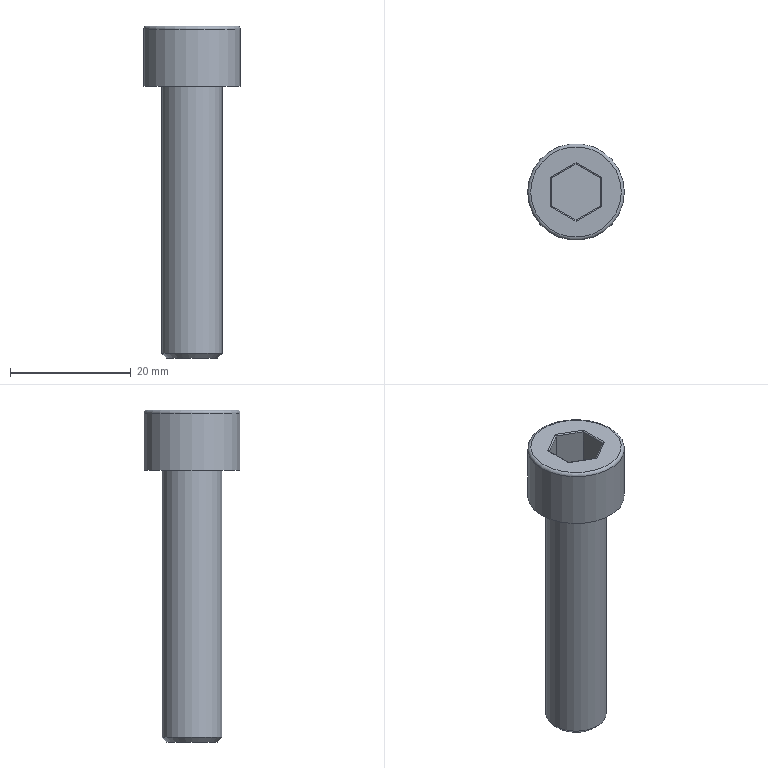Part | STEP file | 200 mesh_id750_x | 1 solid | 20 faces | box 16 x 16 x 55 mm | volume 5201 mm3 | plane 10 | cylinder 8 | torus 1 | cone 1 | commonest cylinder face diameters 0.4 x6 10 x1 16 x1
STEP:
#1=CARTESIAN_POINT('',(-17147.884,-4090.119,38.));
#2=VERTEX_POINT('',#1);
#3=CARTESIAN_POINT('',(-17152.084,-4087.694,38.));
#4=VERTEX_POINT('',#3);
#5=CARTESIAN_POINT('',(-17149.984,-4088.906,38.));
#6=DIRECTION('',(-0.866,0.5,0.));
#7=VECTOR('',#6,1.);
#8=LINE('',#5,#7);
#9=EDGE_CURVE('',#2,#4,#8,.T.);
#10=ORIENTED_EDGE('',*,*,#9,.T.);
#11=CARTESIAN_POINT('',(-17152.084,-4082.844,38.));
#12=VERTEX_POINT('',#11);
#13=CARTESIAN_POINT('',(-17152.084,-4085.269,38.));
#14=DIRECTION('',(0.,1.,0.));
#15=VECTOR('',#14,1.);
#16=LINE('',#13,#15);
#17=EDGE_CURVE('',#4,#12,#16,.T.);
#18=ORIENTED_EDGE('',*,*,#17,.T.);
#19=CARTESIAN_POINT('',(-17147.884,-4080.419,38.));
#20=VERTEX_POINT('',#19);
#21=CARTESIAN_POINT('',(-17149.984,-4081.632,38.));
#22=DIRECTION('',(0.866,0.5,0.));
#23=VECTOR('',#22,1.);
#24=LINE('',#21,#23);
#25=EDGE_CURVE('',#12,#20,#24,.T.);
#26=ORIENTED_EDGE('',*,*,#25,.T.);
#27=CARTESIAN_POINT('',(-17143.684,-4082.844,38.));
#28=VERTEX_POINT('',#27);
#29=CARTESIAN_POINT('',(-17145.784,-4081.632,38.));
#30=DIRECTION('',(0.866,-0.5,0.));
#31=VECTOR('',#30,1.);
#32=LINE('',#29,#31);
#33=EDGE_CURVE('',#20,#28,#32,.T.);
#34=ORIENTED_EDGE('',*,*,#33,.T.);
#35=CARTESIAN_POINT('',(-17143.684,-4087.694,38.));
#36=VERTEX_POINT('',#35);
#37=CARTESIAN_POINT('',(-17143.684,-4085.269,38.));
#38=DIRECTION('',(0.,-1.,0.));
#39=VECTOR('',#38,1.);
#40=LINE('',#37,#39);
#41=EDGE_CURVE('',#28,#36,#40,.T.);
#42=ORIENTED_EDGE('',*,*,#41,.T.);
#43=CARTESIAN_POINT('',(-17145.784,-4088.906,38.));
#44=DIRECTION('',(-0.866,-0.5,0.));
#45=VECTOR('',#44,1.);
#46=LINE('',#43,#45);
#47=EDGE_CURVE('',#36,#2,#46,.T.);
#48=ORIENTED_EDGE('',*,*,#47,.T.);
#49=EDGE_LOOP('',(#10,#18,#26,#34,#42,#48));
#50=FACE_BOUND('',#49,.T.);
#51=CARTESIAN_POINT('',(-17140.384,-4085.269,38.));
#52=VERTEX_POINT('',#51);
#53=CARTESIAN_POINT('',(-17147.884,-4085.269,38.));
#54=DIRECTION('',(0.,0.,1.));
#55=DIRECTION('',(1.,0.,0.));
#56=AXIS2_PLACEMENT_3D('',#53,#54,#55);
#57=CIRCLE('',#56,7.5);
#58=EDGE_CURVE('',#52,#52,#57,.T.);
#59=ORIENTED_EDGE('',*,*,#58,.T.);
#60=EDGE_LOOP('',(#59));
#61=FACE_BOUND('',#60,.T.);
#62=CARTESIAN_POINT('',(-17147.884,-4085.269,38.));
#63=DIRECTION('',(0.,0.,1.));
#64=DIRECTION('',(1.,0.,0.));
#65=AXIS2_PLACEMENT_3D('',#62,#63,#64);
#66=PLANE('',#65);
#67=ADVANCED_FACE('',(#50,#61),#66,.T.);
#68=CARTESIAN_POINT('',(-17152.884,-4085.269,-16.25));
#69=VERTEX_POINT('',#68);
#70=CARTESIAN_POINT('',(-17147.884,-4085.269,-16.25));
#71=DIRECTION('',(0.,0.,1.));
#72=DIRECTION('',(-1.,0.,0.));
#73=AXIS2_PLACEMENT_3D('',#70,#71,#72);
#74=CIRCLE('',#73,5.);
#75=EDGE_CURVE('',#69,#69,#74,.T.);
#76=ORIENTED_EDGE('',*,*,#75,.T.);
#77=EDGE_LOOP('',(#76));
#78=FACE_BOUND('',#77,.T.);
#79=CARTESIAN_POINT('',(-17152.884,-4085.269,28.));
#80=VERTEX_POINT('',#79);
#81=CARTESIAN_POINT('',(-17147.884,-4085.269,28.));
#82=DIRECTION('',(0.,0.,1.));
#83=DIRECTION('',(-1.,0.,0.));
#84=AXIS2_PLACEMENT_3D('',#81,#82,#83);
#85=CIRCLE('',#84,5.);
#86=EDGE_CURVE('',#80,#80,#85,.T.);
#87=ORIENTED_EDGE('',*,*,#86,.F.);
#88=EDGE_LOOP('',(#87));
#89=FACE_BOUND('',#88,.T.);
#90=CARTESIAN_POINT('',(-17147.884,-4085.269,28.));
#91=DIRECTION('',(0.,0.,-1.));
#92=DIRECTION('',(1.,0.,0.));
#93=AXIS2_PLACEMENT_3D('',#90,#91,#92);
#94=CYLINDRICAL_SURFACE('',#93,5.);
#95=ADVANCED_FACE('',(#78,#89),#94,.T.);
#96=ORIENTED_EDGE('',*,*,#86,.T.);
#97=EDGE_LOOP('',(#96));
#98=FACE_BOUND('',#97,.T.);
#99=CARTESIAN_POINT('',(-17139.884,-4085.269,28.));
#100=VERTEX_POINT('',#99);
#101=CARTESIAN_POINT('',(-17147.884,-4085.269,28.));
#102=DIRECTION('',(0.,0.,1.));
#103=DIRECTION('',(1.,0.,0.));
#104=AXIS2_PLACEMENT_3D('',#101,#102,#103);
#105=CIRCLE('',#104,8.);
#106=EDGE_CURVE('',#100,#100,#105,.T.);
#107=ORIENTED_EDGE('',*,*,#106,.F.);
#108=EDGE_LOOP('',(#107));
#109=FACE_BOUND('',#108,.T.);
#110=CARTESIAN_POINT('',(-17147.884,-4085.269,28.));
#111=DIRECTION('',(0.,0.,-1.));
#112=DIRECTION('',(-1.,0.,0.));
#113=AXIS2_PLACEMENT_3D('',#110,#111,#112);
#114=PLANE('',#113);
#115=ADVANCED_FACE('',(#98,#109),#114,.T.);
#116=CARTESIAN_POINT('',(-17139.884,-4085.269,37.5));
#117=VERTEX_POINT('',#116);
#118=CARTESIAN_POINT('',(-17147.884,-4085.269,37.5));
#119=DIRECTION('',(0.,0.,-1.));
#120=DIRECTION('',(1.,0.,0.));
#121=AXIS2_PLACEMENT_3D('',#118,#119,#120);
#122=CIRCLE('',#121,8.);
#123=EDGE_CURVE('',#117,#117,#122,.T.);
#124=ORIENTED_EDGE('',*,*,#123,.T.);
#125=EDGE_LOOP('',(#124));
#126=FACE_BOUND('',#125,.T.);
#127=ORIENTED_EDGE('',*,*,#106,.T.);
#128=EDGE_LOOP('',(#127));
#129=FACE_BOUND('',#128,.T.);
#130=CARTESIAN_POINT('',(-17147.884,-4085.269,28.));
#131=DIRECTION('',(0.,0.,1.));
#132=DIRECTION('',(1.,0.,0.));
#133=AXIS2_PLACEMENT_3D('',#130,#131,#132);
#134=CYLINDRICAL_SURFACE('',#133,8.);
#135=ADVANCED_FACE('',(#126,#129),#134,.T.);
#136=ORIENTED_EDGE('',*,*,#58,.F.);
#137=EDGE_LOOP('',(#136));
#138=FACE_BOUND('',#137,.T.);
#139=ORIENTED_EDGE('',*,*,#123,.F.);
#140=EDGE_LOOP('',(#139));
#141=FACE_BOUND('',#140,.T.);
#142=CARTESIAN_POINT('',(-17147.884,-4085.269,37.5));
#143=DIRECTION('',(0.,0.,1.));
#144=DIRECTION('',(1.,0.,0.));
#145=AXIS2_PLACEMENT_3D('',#142,#143,#144);
#146=TOROIDAL_SURFACE('',#145,7.5,0.5);
#147=ADVANCED_FACE('',(#138,#141),#146,.T.);
#148=CARTESIAN_POINT('',(-17147.884,-4080.65,37.8));
#149=VERTEX_POINT('',#148);
#150=CARTESIAN_POINT('',(-17147.884,-4080.65,32.));
#151=VERTEX_POINT('',#150);
#152=CARTESIAN_POINT('',(-17147.884,-4080.65,32.));
#153=DIRECTION('',(0.,0.,-1.));
#154=VECTOR('',#153,1.);
#155=LINE('',#152,#154);
#156=EDGE_CURVE('',#149,#151,#155,.T.);
#157=ORIENTED_EDGE('',*,*,#156,.F.);
#158=CARTESIAN_POINT('',(-17151.884,-4082.96,37.8));
#159=VERTEX_POINT('',#158);
#160=CARTESIAN_POINT('',(-17151.884,-4082.96,37.8));
#161=DIRECTION('',(-0.866,-0.5,0.));
#162=VECTOR('',#161,1.);
#163=LINE('',#160,#162);
#164=EDGE_CURVE('',#149,#159,#163,.T.);
#165=ORIENTED_EDGE('',*,*,#164,.T.);
#166=CARTESIAN_POINT('',(-17151.884,-4082.96,32.));
#167=VERTEX_POINT('',#166);
#168=CARTESIAN_POINT('',(-17151.884,-4082.96,32.));
#169=DIRECTION('',(0.,0.,-1.));
#170=VECTOR('',#169,1.);
#171=LINE('',#168,#170);
#172=EDGE_CURVE('',#159,#167,#171,.T.);
#173=ORIENTED_EDGE('',*,*,#172,.T.);
#174=CARTESIAN_POINT('',(-17151.884,-4082.96,32.));
#175=DIRECTION('',(-0.866,-0.5,0.));
#176=VECTOR('',#175,1.);
#177=LINE('',#174,#176);
#178=EDGE_CURVE('',#151,#167,#177,.T.);
#179=ORIENTED_EDGE('',*,*,#178,.F.);
#180=EDGE_LOOP('',(#157,#165,#173,#179));
#181=FACE_OUTER_BOUND('',#180,.T.);
#182=CARTESIAN_POINT('',(-17151.884,-4082.96,32.));
#183=DIRECTION('',(0.5,-0.866,0.));
#184=DIRECTION('',(0.866,0.5,0.));
#185=AXIS2_PLACEMENT_3D('',#182,#183,#184);
#186=PLANE('',#185);
#187=ADVANCED_FACE('',(#181),#186,.T.);
#188=CARTESIAN_POINT('',(-17143.884,-4082.96,37.8));
#189=VERTEX_POINT('',#188);
#190=CARTESIAN_POINT('',(-17143.884,-4082.96,32.));
#191=VERTEX_POINT('',#190);
#192=CARTESIAN_POINT('',(-17143.884,-4082.96,32.));
#193=DIRECTION('',(0.,0.,-1.));
#194=VECTOR('',#193,1.);
#195=LINE('',#192,#194);
#196=EDGE_CURVE('',#189,#191,#195,.T.);
#197=ORIENTED_EDGE('',*,*,#196,.F.);
#198=CARTESIAN_POINT('',(-17147.884,-4080.65,37.8));
#199=DIRECTION('',(-0.866,0.5,0.));
#200=VECTOR('',#199,1.);
#201=LINE('',#198,#200);
#202=EDGE_CURVE('',#189,#149,#201,.T.);
#203=ORIENTED_EDGE('',*,*,#202,.T.);
#204=ORIENTED_EDGE('',*,*,#156,.T.);
#205=CARTESIAN_POINT('',(-17147.884,-4080.65,32.));
#206=DIRECTION('',(-0.866,0.5,0.));
#207=VECTOR('',#206,1.);
#208=LINE('',#205,#207);
#209=EDGE_CURVE('',#191,#151,#208,.T.);
#210=ORIENTED_EDGE('',*,*,#209,.F.);
#211=EDGE_LOOP('',(#197,#203,#204,#210));
#212=FACE_OUTER_BOUND('',#211,.T.);
#213=CARTESIAN_POINT('',(-17147.884,-4080.65,32.));
#214=DIRECTION('',(-0.5,-0.866,0.));
#215=DIRECTION('',(0.866,-0.5,0.));
#216=AXIS2_PLACEMENT_3D('',#213,#214,#215);
#217=PLANE('',#216);
#218=ADVANCED_FACE('',(#212),#217,.T.);
#219=CARTESIAN_POINT('',(-17143.884,-4087.579,37.8));
#220=VERTEX_POINT('',#219);
#221=CARTESIAN_POINT('',(-17143.884,-4087.579,32.));
#222=VERTEX_POINT('',#221);
#223=CARTESIAN_POINT('',(-17143.884,-4087.579,32.));
#224=DIRECTION('',(0.,0.,-1.));
#225=VECTOR('',#224,1.);
#226=LINE('',#223,#225);
#227=EDGE_CURVE('',#220,#222,#226,.T.);
#228=ORIENTED_EDGE('',*,*,#227,.F.);
#229=CARTESIAN_POINT('',(-17143.884,-4082.96,37.8));
#230=DIRECTION('',(0.,1.,0.));
#231=VECTOR('',#230,1.);
#232=LINE('',#229,#231);
#233=EDGE_CURVE('',#220,#189,#232,.T.);
#234=ORIENTED_EDGE('',*,*,#233,.T.);
#235=ORIENTED_EDGE('',*,*,#196,.T.);
#236=CARTESIAN_POINT('',(-17143.884,-4082.96,32.));
#237=DIRECTION('',(0.,1.,0.));
#238=VECTOR('',#237,1.);
#239=LINE('',#236,#238);
#240=EDGE_CURVE('',#222,#191,#239,.T.);
#241=ORIENTED_EDGE('',*,*,#240,.F.);
#242=EDGE_LOOP('',(#228,#234,#235,#241));
#243=FACE_OUTER_BOUND('',#242,.T.);
#244=CARTESIAN_POINT('',(-17143.884,-4082.96,32.));
#245=DIRECTION('',(-1.,0.,0.));
#246=DIRECTION('',(0.,0.,1.));
#247=AXIS2_PLACEMENT_3D('',#244,#245,#246);
#248=PLANE('',#247);
#249=ADVANCED_FACE('',(#243),#248,.T.);
#250=CARTESIAN_POINT('',(-17147.884,-4089.888,37.8));
#251=VERTEX_POINT('',#250);
#252=CARTESIAN_POINT('',(-17147.884,-4089.888,32.));
#253=VERTEX_POINT('',#252);
#254=CARTESIAN_POINT('',(-17147.884,-4089.888,32.));
#255=DIRECTION('',(0.,0.,-1.));
#256=VECTOR('',#255,1.);
#257=LINE('',#254,#256);
#258=EDGE_CURVE('',#251,#253,#257,.T.);
#259=ORIENTED_EDGE('',*,*,#258,.F.);
#260=CARTESIAN_POINT('',(-17143.884,-4087.579,37.8));
#261=DIRECTION('',(0.866,0.5,0.));
#262=VECTOR('',#261,1.);
#263=LINE('',#260,#262);
#264=EDGE_CURVE('',#251,#220,#263,.T.);
#265=ORIENTED_EDGE('',*,*,#264,.T.);
#266=ORIENTED_EDGE('',*,*,#227,.T.);
#267=CARTESIAN_POINT('',(-17143.884,-4087.579,32.));
#268=DIRECTION('',(0.866,0.5,0.));
#269=VECTOR('',#268,1.);
#270=LINE('',#267,#269);
#271=EDGE_CURVE('',#253,#222,#270,.T.);
#272=ORIENTED_EDGE('',*,*,#271,.F.);
#273=EDGE_LOOP('',(#259,#265,#266,#272));
#274=FACE_OUTER_BOUND('',#273,.T.);
#275=CARTESIAN_POINT('',(-17143.884,-4087.579,32.));
#276=DIRECTION('',(-0.5,0.866,0.));
#277=DIRECTION('',(-0.866,-0.5,0.));
#278=AXIS2_PLACEMENT_3D('',#275,#276,#277);
#279=PLANE('',#278);
#280=ADVANCED_FACE('',(#274),#279,.T.);
#281=CARTESIAN_POINT('',(-17151.884,-4087.579,37.8));
#282=VERTEX_POINT('',#281);
#283=CARTESIAN_POINT('',(-17151.884,-4087.579,32.));
#284=VERTEX_POINT('',#283);
#285=CARTESIAN_POINT('',(-17151.884,-4087.579,32.));
#286=DIRECTION('',(0.,0.,-1.));
#287=VECTOR('',#286,1.);
#288=LINE('',#285,#287);
#289=EDGE_CURVE('',#282,#284,#288,.T.);
#290=ORIENTED_EDGE('',*,*,#289,.F.);
#291=CARTESIAN_POINT('',(-17147.884,-4089.888,37.8));
#292=DIRECTION('',(0.866,-0.5,0.));
#293=VECTOR('',#292,1.);
#294=LINE('',#291,#293);
#295=EDGE_CURVE('',#282,#251,#294,.T.);
#296=ORIENTED_EDGE('',*,*,#295,.T.);
#297=ORIENTED_EDGE('',*,*,#258,.T.);
#298=CARTESIAN_POINT('',(-17147.884,-4089.888,32.));
#299=DIRECTION('',(0.866,-0.5,0.));
#300=VECTOR('',#299,1.);
#301=LINE('',#298,#300);
#302=EDGE_CURVE('',#284,#253,#301,.T.);
#303=ORIENTED_EDGE('',*,*,#302,.F.);
#304=EDGE_LOOP('',(#290,#296,#297,#303));
#305=FACE_OUTER_BOUND('',#304,.T.);
#306=CARTESIAN_POINT('',(-17147.884,-4089.888,32.));
#307=DIRECTION('',(0.5,0.866,0.));
#308=DIRECTION('',(-0.866,0.5,0.));
#309=AXIS2_PLACEMENT_3D('',#306,#307,#308);
#310=PLANE('',#309);
#311=ADVANCED_FACE('',(#305),#310,.T.);
#312=ORIENTED_EDGE('',*,*,#172,.F.);
#313=CARTESIAN_POINT('',(-17151.884,-4087.579,37.8));
#314=DIRECTION('',(0.,-1.,0.));
#315=VECTOR('',#314,1.);
#316=LINE('',#313,#315);
#317=EDGE_CURVE('',#159,#282,#316,.T.);
#318=ORIENTED_EDGE('',*,*,#317,.T.);
#319=ORIENTED_EDGE('',*,*,#289,.T.);
#320=CARTESIAN_POINT('',(-17151.884,-4087.579,32.));
#321=DIRECTION('',(0.,-1.,0.));
#322=VECTOR('',#321,1.);
#323=LINE('',#320,#322);
#324=EDGE_CURVE('',#167,#284,#323,.T.);
#325=ORIENTED_EDGE('',*,*,#324,.F.);
#326=EDGE_LOOP('',(#312,#318,#319,#325));
#327=FACE_OUTER_BOUND('',#326,.T.);
#328=CARTESIAN_POINT('',(-17151.884,-4087.579,32.));
#329=DIRECTION('',(1.,0.,0.));
#330=DIRECTION('',(0.,0.,-1.));
#331=AXIS2_PLACEMENT_3D('',#328,#329,#330);
#332=PLANE('',#331);
#333=ADVANCED_FACE('',(#327),#332,.T.);
#334=ORIENTED_EDGE('',*,*,#178,.T.);
#335=ORIENTED_EDGE('',*,*,#324,.T.);
#336=ORIENTED_EDGE('',*,*,#302,.T.);
#337=ORIENTED_EDGE('',*,*,#271,.T.);
#338=ORIENTED_EDGE('',*,*,#240,.T.);
#339=ORIENTED_EDGE('',*,*,#209,.T.);
#340=EDGE_LOOP('',(#334,#335,#336,#337,#338,#339));
#341=FACE_OUTER_BOUND('',#340,.T.);
#342=CARTESIAN_POINT('',(0.,0.,32.));
#343=DIRECTION('',(0.,0.,-1.));
#344=DIRECTION('',(-1.,0.,0.));
#345=AXIS2_PLACEMENT_3D('',#342,#343,#344);
#346=PLANE('',#345);
#347=ADVANCED_FACE('',(#341),#346,.F.);
#348=CARTESIAN_POINT('',(-17143.684,-4082.844,37.8));
#349=DIRECTION('',(-0.5,0.866,0.));
#350=DIRECTION('',(0.866,0.5,0.));
#351=AXIS2_PLACEMENT_3D('',#348,#349,#350);
#352=ELLIPSE('',#351,0.2309,0.2);
#353=EDGE_CURVE('',#189,#28,#352,.T.);
#354=ORIENTED_EDGE('',*,*,#353,.F.);
#355=ORIENTED_EDGE('',*,*,#233,.F.);
#356=CARTESIAN_POINT('',(-17143.684,-4087.694,37.8));
#357=DIRECTION('',(-0.5,-0.866,0.));
#358=DIRECTION('',(0.866,-0.5,0.));
#359=AXIS2_PLACEMENT_3D('',#356,#357,#358);
#360=ELLIPSE('',#359,0.2309,0.2);
#361=EDGE_CURVE('',#36,#220,#360,.T.);
#362=ORIENTED_EDGE('',*,*,#361,.F.);
#363=ORIENTED_EDGE('',*,*,#41,.F.);
#364=EDGE_LOOP('',(#354,#355,#362,#363));
#365=FACE_OUTER_BOUND('',#364,.T.);
#366=CARTESIAN_POINT('',(-17143.684,-4085.269,37.8));
#367=DIRECTION('',(0.,-1.,0.));
#368=DIRECTION('',(0.,0.,-1.));
#369=AXIS2_PLACEMENT_3D('',#366,#367,#368);
#370=CYLINDRICAL_SURFACE('',#369,0.2);
#371=ADVANCED_FACE('',(#365),#370,.T.);
#372=ORIENTED_EDGE('',*,*,#361,.T.);
#373=ORIENTED_EDGE('',*,*,#264,.F.);
#374=CARTESIAN_POINT('',(-17147.884,-4090.119,37.8));
#375=DIRECTION('',(-1.,0.,0.));
#376=DIRECTION('',(0.,-1.,0.));
#377=AXIS2_PLACEMENT_3D('',#374,#375,#376);
#378=ELLIPSE('',#377,0.2309,0.2);
#379=EDGE_CURVE('',#2,#251,#378,.T.);
#380=ORIENTED_EDGE('',*,*,#379,.F.);
#381=ORIENTED_EDGE('',*,*,#47,.F.);
#382=EDGE_LOOP('',(#372,#373,#380,#381));
#383=FACE_OUTER_BOUND('',#382,.T.);
#384=CARTESIAN_POINT('',(-17145.784,-4088.906,37.8));
#385=DIRECTION('',(-0.866,-0.5,0.));
#386=DIRECTION('',(0.5,-0.866,0.));
#387=AXIS2_PLACEMENT_3D('',#384,#385,#386);
#388=CYLINDRICAL_SURFACE('',#387,0.2);
#389=ADVANCED_FACE('',(#383),#388,.T.);
#390=ORIENTED_EDGE('',*,*,#353,.T.);
#391=ORIENTED_EDGE('',*,*,#33,.F.);
#392=CARTESIAN_POINT('',(-17147.884,-4080.419,37.8));
#393=DIRECTION('',(-1.,0.,0.));
#394=DIRECTION('',(0.,1.,0.));
#395=AXIS2_PLACEMENT_3D('',#392,#393,#394);
#396=ELLIPSE('',#395,0.2309,0.2);
#397=EDGE_CURVE('',#149,#20,#396,.T.);
#398=ORIENTED_EDGE('',*,*,#397,.F.);
#399=ORIENTED_EDGE('',*,*,#202,.F.);
#400=EDGE_LOOP('',(#390,#391,#398,#399));
#401=FACE_OUTER_BOUND('',#400,.T.);
#402=CARTESIAN_POINT('',(-17145.784,-4081.632,37.8));
#403=DIRECTION('',(0.866,-0.5,0.));
#404=DIRECTION('',(0.5,0.866,0.));
#405=AXIS2_PLACEMENT_3D('',#402,#403,#404);
#406=CYLINDRICAL_SURFACE('',#405,0.2);
#407=ADVANCED_FACE('',(#401),#406,.T.);
#408=ORIENTED_EDGE('',*,*,#379,.T.);
#409=ORIENTED_EDGE('',*,*,#295,.F.);
#410=CARTESIAN_POINT('',(-17152.084,-4087.694,37.8));
#411=DIRECTION('',(-0.5,0.866,0.));
#412=DIRECTION('',(0.866,0.5,0.));
#413=AXIS2_PLACEMENT_3D('',#410,#411,#412);
#414=ELLIPSE('',#413,0.2309,0.2);
#415=EDGE_CURVE('',#4,#282,#414,.T.);
#416=ORIENTED_EDGE('',*,*,#415,.F.);
#417=ORIENTED_EDGE('',*,*,#9,.F.);
#418=EDGE_LOOP('',(#408,#409,#416,#417));
#419=FACE_OUTER_BOUND('',#418,.T.);
#420=CARTESIAN_POINT('',(-17149.984,-4088.906,37.8));
#421=DIRECTION('',(-0.866,0.5,0.));
#422=DIRECTION('',(-0.5,-0.866,0.));
#423=AXIS2_PLACEMENT_3D('',#420,#421,#422);
#424=CYLINDRICAL_SURFACE('',#423,0.2);
#425=ADVANCED_FACE('',(#419),#424,.T.);
#426=ORIENTED_EDGE('',*,*,#397,.T.);
#427=ORIENTED_EDGE('',*,*,#25,.F.);
#428=CARTESIAN_POINT('',(-17152.084,-4082.844,37.8));
#429=DIRECTION('',(-0.5,-0.866,0.));
#430=DIRECTION('',(-0.866,0.5,0.));
#431=AXIS2_PLACEMENT_3D('',#428,#429,#430);
#432=ELLIPSE('',#431,0.2309,0.2);
#433=EDGE_CURVE('',#159,#12,#432,.T.);
#434=ORIENTED_EDGE('',*,*,#433,.F.);
#435=ORIENTED_EDGE('',*,*,#164,.F.);
#436=EDGE_LOOP('',(#426,#427,#434,#435));
#437=FACE_OUTER_BOUND('',#436,.T.);
#438=CARTESIAN_POINT('',(-17149.984,-4081.632,37.8));
#439=DIRECTION('',(0.866,0.5,0.));
#440=DIRECTION('',(-0.5,0.866,0.));
#441=AXIS2_PLACEMENT_3D('',#438,#439,#440);
#442=CYLINDRICAL_SURFACE('',#441,0.2);
#443=ADVANCED_FACE('',(#437),#442,.T.);
#444=ORIENTED_EDGE('',*,*,#415,.T.);
#445=ORIENTED_EDGE('',*,*,#317,.F.);
#446=ORIENTED_EDGE('',*,*,#433,.T.);
#447=ORIENTED_EDGE('',*,*,#17,.F.);
#448=EDGE_LOOP('',(#444,#445,#446,#447));
#449=FACE_OUTER_BOUND('',#448,.T.);
#450=CARTESIAN_POINT('',(-17152.084,-4085.269,37.8));
#451=DIRECTION('',(0.,1.,0.));
#452=DIRECTION('',(0.,0.,1.));
#453=AXIS2_PLACEMENT_3D('',#450,#451,#452);
#454=CYLINDRICAL_SURFACE('',#453,0.2);
#455=ADVANCED_FACE('',(#449),#454,.T.);
#456=CARTESIAN_POINT('',(-17152.134,-4085.269,-17.));
#457=VERTEX_POINT('',#456);
#458=CARTESIAN_POINT('',(-17147.884,-4085.269,-17.));
#459=DIRECTION('',(0.,0.,-1.));
#460=DIRECTION('',(-1.,0.,0.));
#461=AXIS2_PLACEMENT_3D('',#458,#459,#460);
#462=CIRCLE('',#461,4.25);
#463=EDGE_CURVE('',#457,#457,#462,.T.);
#464=ORIENTED_EDGE('',*,*,#463,.T.);
#465=EDGE_LOOP('',(#464));
#466=FACE_OUTER_BOUND('',#465,.T.);
#467=CARTESIAN_POINT('',(-17147.884,-4085.269,-17.));
#468=DIRECTION('',(0.,0.,-1.));
#469=DIRECTION('',(-1.,0.,0.));
#470=AXIS2_PLACEMENT_3D('',#467,#468,#469);
#471=PLANE('',#470);
#472=ADVANCED_FACE('',(#466),#471,.T.);
#473=ORIENTED_EDGE('',*,*,#463,.F.);
#474=EDGE_LOOP('',(#473));
#475=FACE_BOUND('',#474,.T.);
#476=ORIENTED_EDGE('',*,*,#75,.F.);
#477=EDGE_LOOP('',(#476));
#478=FACE_BOUND('',#477,.T.);
#479=CARTESIAN_POINT('',(-17147.884,-4085.269,-16.25));
#480=DIRECTION('',(0.,0.,1.));
#481=DIRECTION('',(1.,0.,0.));
#482=AXIS2_PLACEMENT_3D('',#479,#480,#481);
#483=CONICAL_SURFACE('',#482,5.,45.);
#484=ADVANCED_FACE('',(#475,#478),#483,.T.);
#485=CLOSED_SHELL('',(#67,#95,#115,#135,#147,#187,#218,#249,#280,#311,#333,#347,#371,#389,#407,#425,#443,#455,#472,#484));
#486=MANIFOLD_SOLID_BREP('',#485);
#487=(LENGTH_UNIT()NAMED_UNIT(*)SI_UNIT(.MILLI.,.METRE.));
#488=UNCERTAINTY_MEASURE_WITH_UNIT(LENGTH_MEASURE(0.00002),#487,'','');
#489=(NAMED_UNIT(*)PLANE_ANGLE_UNIT()SI_UNIT($,.RADIAN.));
#490=PLANE_ANGLE_MEASURE_WITH_UNIT(PLANE_ANGLE_MEASURE(0.01745),#489);
#491=DIMENSIONAL_EXPONENTS(0.,0.,0.,0.,0.,0.,0.);
#492=(CONVERSION_BASED_UNIT('DEGREE',#490)NAMED_UNIT(#491)PLANE_ANGLE_UNIT());
#493=(NAMED_UNIT(*)SI_UNIT($,.STERADIAN.)SOLID_ANGLE_UNIT());
#494=(GEOMETRIC_REPRESENTATION_CONTEXT(3)GLOBAL_UNCERTAINTY_ASSIGNED_CONTEXT((#488))GLOBAL_UNIT_ASSIGNED_CONTEXT((#487,#492,#493))REPRESENTATION_CONTEXT('',''));
#495=ADVANCED_BREP_SHAPE_REPRESENTATION('',(#486),#494);